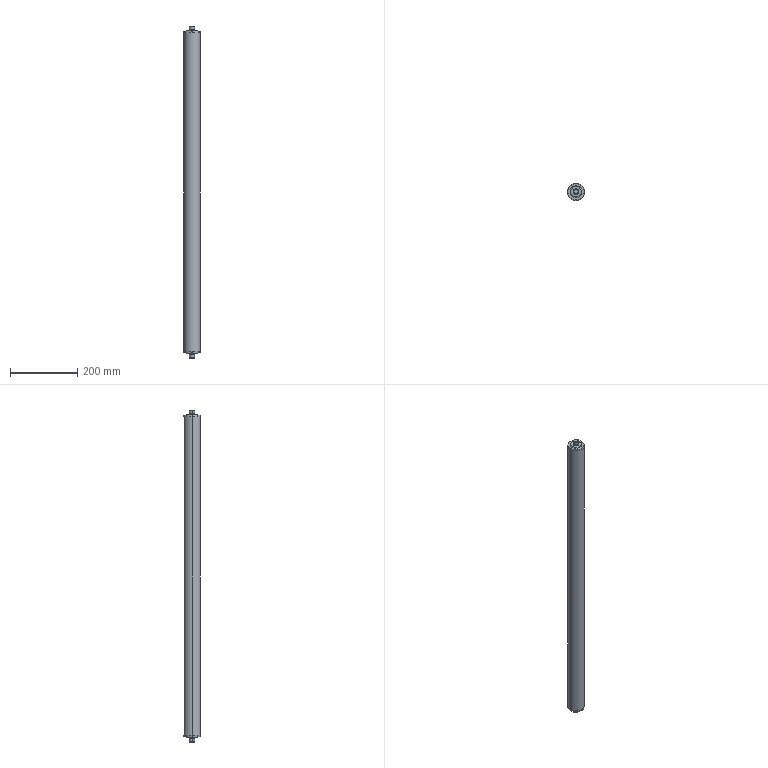Part | SolidWorks | features Chamfer 2, ICE 2, Revolution 1 | 1 solid | 30 faces | box 50 x 50 x 985 mm | volume 1880684 mm3 | cone 12 | cylinder 10 | plane 8 | commonest cylinder face diameters 15 x4 17 x4 50 x2
STEP:
#1=CARTESIAN_POINT('',(6.5,0.,340.5));
#2=VERTEX_POINT('',#1);
#3=CARTESIAN_POINT('',(-6.5,0.,340.5));
#4=VERTEX_POINT('',#3);
#5=CARTESIAN_POINT('',(0.,0.,340.5));
#6=DIRECTION('',(0.,0.,1.));
#7=DIRECTION('',(-1.,0.,0.));
#8=AXIS2_PLACEMENT_3D('',#5,#6,#7);
#9=CIRCLE('',#8,6.5);
#10=EDGE_CURVE('',#2,#4,#9,.T.);
#11=ORIENTED_EDGE('',*,*,#10,.F.);
#12=CARTESIAN_POINT('',(7.5,0.,339.5));
#13=VERTEX_POINT('',#12);
#14=CARTESIAN_POINT('',(6.5,0.,340.5));
#15=DIRECTION('',(0.7071,0.,-0.7071));
#16=VECTOR('',#15,1000.);
#17=LINE('',#14,#16);
#18=EDGE_CURVE('',#2,#13,#17,.T.);
#19=ORIENTED_EDGE('',*,*,#18,.T.);
#20=CARTESIAN_POINT('',(-7.5,0.,339.5));
#21=VERTEX_POINT('',#20);
#22=CARTESIAN_POINT('',(0.,0.,339.5));
#23=DIRECTION('',(0.,0.,-1.));
#24=DIRECTION('',(-1.,0.,0.));
#25=AXIS2_PLACEMENT_3D('',#22,#23,#24);
#26=CIRCLE('',#25,7.5);
#27=EDGE_CURVE('',#21,#13,#26,.T.);
#28=ORIENTED_EDGE('',*,*,#27,.F.);
#29=CARTESIAN_POINT('',(-6.5,0.,340.5));
#30=DIRECTION('',(-0.7071,0.,-0.7071));
#31=VECTOR('',#30,1000.);
#32=LINE('',#29,#31);
#33=EDGE_CURVE('',#4,#21,#32,.T.);
#34=ORIENTED_EDGE('',*,*,#33,.F.);
#35=EDGE_LOOP('',(#11,#19,#28,#34));
#36=FACE_OUTER_BOUND('',#35,.T.);
#37=CARTESIAN_POINT('',(0.,0.,340.5));
#38=DIRECTION('',(0.,0.,-1.));
#39=DIRECTION('',(-1.,0.,0.));
#40=AXIS2_PLACEMENT_3D('',#37,#38,#39);
#41=CONICAL_SURFACE('',#40,6.5,0.7854);
#42=ADVANCED_FACE('',(#36),#41,.T.);
#43=CARTESIAN_POINT('',(-6.5,0.,-644.5));
#44=VERTEX_POINT('',#43);
#45=CARTESIAN_POINT('',(6.5,0.,-644.5));
#46=VERTEX_POINT('',#45);
#47=CARTESIAN_POINT('',(0.,0.,-644.5));
#48=DIRECTION('',(0.,0.,-1.));
#49=DIRECTION('',(1.,0.,0.));
#50=AXIS2_PLACEMENT_3D('',#47,#48,#49);
#51=CIRCLE('',#50,6.5);
#52=EDGE_CURVE('',#44,#46,#51,.T.);
#53=ORIENTED_EDGE('',*,*,#52,.F.);
#54=CARTESIAN_POINT('',(-7.5,0.,-643.5));
#55=VERTEX_POINT('',#54);
#56=CARTESIAN_POINT('',(-7.5,0.,-643.5));
#57=DIRECTION('',(-0.7071,0.,0.7071));
#58=VECTOR('',#57,1000.);
#59=LINE('',#56,#58);
#60=EDGE_CURVE('',#44,#55,#59,.T.);
#61=ORIENTED_EDGE('',*,*,#60,.T.);
#62=CARTESIAN_POINT('',(7.5,0.,-643.5));
#63=VERTEX_POINT('',#62);
#64=CARTESIAN_POINT('',(0.,0.,-643.5));
#65=DIRECTION('',(0.,0.,1.));
#66=DIRECTION('',(1.,0.,0.));
#67=AXIS2_PLACEMENT_3D('',#64,#65,#66);
#68=CIRCLE('',#67,7.5);
#69=EDGE_CURVE('',#63,#55,#68,.T.);
#70=ORIENTED_EDGE('',*,*,#69,.F.);
#71=CARTESIAN_POINT('',(7.5,0.,-643.5));
#72=DIRECTION('',(0.7071,0.,0.7071));
#73=VECTOR('',#72,1000.);
#74=LINE('',#71,#73);
#75=EDGE_CURVE('',#46,#63,#74,.T.);
#76=ORIENTED_EDGE('',*,*,#75,.F.);
#77=EDGE_LOOP('',(#53,#61,#70,#76));
#78=FACE_OUTER_BOUND('',#77,.T.);
#79=CARTESIAN_POINT('',(0.,0.,-643.5));
#80=DIRECTION('',(0.,0.,1.));
#81=DIRECTION('',(1.,0.,0.));
#82=AXIS2_PLACEMENT_3D('',#79,#80,#81);
#83=CONICAL_SURFACE('',#82,7.5,0.7854);
#84=ADVANCED_FACE('',(#78),#83,.T.);
#85=CARTESIAN_POINT('',(24.118,0.,325.));
#86=VERTEX_POINT('',#85);
#87=CARTESIAN_POINT('',(-24.118,0.,325.));
#88=VERTEX_POINT('',#87);
#89=CARTESIAN_POINT('',(0.,0.,325.));
#90=DIRECTION('',(0.,0.,1.));
#91=DIRECTION('',(-1.,0.,0.));
#92=AXIS2_PLACEMENT_3D('',#89,#90,#91);
#93=CIRCLE('',#92,24.118);
#94=EDGE_CURVE('',#86,#88,#93,.T.);
#95=ORIENTED_EDGE('',*,*,#94,.F.);
#96=CARTESIAN_POINT('',(25.,0.,320.));
#97=VERTEX_POINT('',#96);
#98=CARTESIAN_POINT('',(24.118,0.,325.));
#99=DIRECTION('',(0.1736,0.,-0.9848));
#100=VECTOR('',#99,1000.);
#101=LINE('',#98,#100);
#102=EDGE_CURVE('',#86,#97,#101,.T.);
#103=ORIENTED_EDGE('',*,*,#102,.T.);
#104=CARTESIAN_POINT('',(-25.,0.,320.));
#105=VERTEX_POINT('',#104);
#106=CARTESIAN_POINT('',(0.,0.,320.));
#107=DIRECTION('',(0.,0.,-1.));
#108=DIRECTION('',(-1.,0.,0.));
#109=AXIS2_PLACEMENT_3D('',#106,#107,#108);
#110=CIRCLE('',#109,25.);
#111=EDGE_CURVE('',#105,#97,#110,.T.);
#112=ORIENTED_EDGE('',*,*,#111,.F.);
#113=CARTESIAN_POINT('',(-24.118,0.,325.));
#114=DIRECTION('',(-0.1736,0.,-0.9848));
#115=VECTOR('',#114,1000.);
#116=LINE('',#113,#115);
#117=EDGE_CURVE('',#88,#105,#116,.T.);
#118=ORIENTED_EDGE('',*,*,#117,.F.);
#119=EDGE_LOOP('',(#95,#103,#112,#118));
#120=FACE_OUTER_BOUND('',#119,.T.);
#121=CARTESIAN_POINT('',(0.,0.,325.));
#122=DIRECTION('',(0.,0.,-1.));
#123=DIRECTION('',(-1.,0.,0.));
#124=AXIS2_PLACEMENT_3D('',#121,#122,#123);
#125=CONICAL_SURFACE('',#124,24.118,0.1745);
#126=ADVANCED_FACE('',(#120),#125,.T.);
#127=CARTESIAN_POINT('',(-24.118,0.,-629.));
#128=VERTEX_POINT('',#127);
#129=CARTESIAN_POINT('',(24.118,0.,-629.));
#130=VERTEX_POINT('',#129);
#131=CARTESIAN_POINT('',(0.,0.,-629.));
#132=DIRECTION('',(0.,0.,-1.));
#133=DIRECTION('',(1.,0.,0.));
#134=AXIS2_PLACEMENT_3D('',#131,#132,#133);
#135=CIRCLE('',#134,24.118);
#136=EDGE_CURVE('',#128,#130,#135,.T.);
#137=ORIENTED_EDGE('',*,*,#136,.F.);
#138=CARTESIAN_POINT('',(-25.,0.,-624.));
#139=VERTEX_POINT('',#138);
#140=CARTESIAN_POINT('',(-25.,0.,-624.));
#141=DIRECTION('',(-0.1736,0.,0.9848));
#142=VECTOR('',#141,1000.);
#143=LINE('',#140,#142);
#144=EDGE_CURVE('',#128,#139,#143,.T.);
#145=ORIENTED_EDGE('',*,*,#144,.T.);
#146=CARTESIAN_POINT('',(25.,0.,-624.));
#147=VERTEX_POINT('',#146);
#148=CARTESIAN_POINT('',(0.,0.,-624.));
#149=DIRECTION('',(0.,0.,1.));
#150=DIRECTION('',(1.,0.,0.));
#151=AXIS2_PLACEMENT_3D('',#148,#149,#150);
#152=CIRCLE('',#151,25.);
#153=EDGE_CURVE('',#147,#139,#152,.T.);
#154=ORIENTED_EDGE('',*,*,#153,.F.);
#155=CARTESIAN_POINT('',(25.,0.,-624.));
#156=DIRECTION('',(0.1736,0.,0.9848));
#157=VECTOR('',#156,1000.);
#158=LINE('',#155,#157);
#159=EDGE_CURVE('',#130,#147,#158,.T.);
#160=ORIENTED_EDGE('',*,*,#159,.F.);
#161=EDGE_LOOP('',(#137,#145,#154,#160));
#162=FACE_OUTER_BOUND('',#161,.T.);
#163=CARTESIAN_POINT('',(0.,0.,-624.));
#164=DIRECTION('',(0.,0.,1.));
#165=DIRECTION('',(1.,0.,0.));
#166=AXIS2_PLACEMENT_3D('',#163,#164,#165);
#167=CONICAL_SURFACE('',#166,25.,0.1745);
#168=ADVANCED_FACE('',(#162),#167,.T.);
#169=CARTESIAN_POINT('',(15.701,0.,326.761));
#170=VERTEX_POINT('',#169);
#171=CARTESIAN_POINT('',(-15.701,0.,326.761));
#172=VERTEX_POINT('',#171);
#173=CARTESIAN_POINT('',(0.,0.,326.761));
#174=DIRECTION('',(0.,0.,1.));
#175=DIRECTION('',(1.,0.,0.));
#176=AXIS2_PLACEMENT_3D('',#173,#174,#175);
#177=CIRCLE('',#176,15.701);
#178=EDGE_CURVE('',#170,#172,#177,.T.);
#179=ORIENTED_EDGE('',*,*,#178,.F.);
#180=CARTESIAN_POINT('',(17.799,0.,325.));
#181=VERTEX_POINT('',#180);
#182=CARTESIAN_POINT('',(17.799,0.,325.));
#183=DIRECTION('',(0.766,0.,-0.6428));
#184=VECTOR('',#183,1000.);
#185=LINE('',#182,#184);
#186=EDGE_CURVE('',#170,#181,#185,.T.);
#187=ORIENTED_EDGE('',*,*,#186,.T.);
#188=CARTESIAN_POINT('',(-17.799,0.,325.));
#189=VERTEX_POINT('',#188);
#190=CARTESIAN_POINT('',(0.,0.,325.));
#191=DIRECTION('',(0.,0.,1.));
#192=DIRECTION('',(1.,0.,0.));
#193=AXIS2_PLACEMENT_3D('',#190,#191,#192);
#194=CIRCLE('',#193,17.799);
#195=EDGE_CURVE('',#181,#189,#194,.T.);
#196=ORIENTED_EDGE('',*,*,#195,.T.);
#197=CARTESIAN_POINT('',(-17.799,0.,325.));
#198=DIRECTION('',(-0.766,0.,-0.6428));
#199=VECTOR('',#198,1000.);
#200=LINE('',#197,#199);
#201=EDGE_CURVE('',#172,#189,#200,.T.);
#202=ORIENTED_EDGE('',*,*,#201,.F.);
#203=EDGE_LOOP('',(#179,#187,#196,#202));
#204=FACE_OUTER_BOUND('',#203,.T.);
#205=CARTESIAN_POINT('',(0.,0.,325.));
#206=DIRECTION('',(0.,0.,-1.));
#207=DIRECTION('',(-1.,0.,0.));
#208=AXIS2_PLACEMENT_3D('',#205,#206,#207);
#209=CONICAL_SURFACE('',#208,17.799,0.8727);
#210=ADVANCED_FACE('',(#204),#209,.T.);
#211=CARTESIAN_POINT('',(8.5,0.,326.761));
#212=VERTEX_POINT('',#211);
#213=CARTESIAN_POINT('',(-8.5,0.,326.761));
#214=VERTEX_POINT('',#213);
#215=CARTESIAN_POINT('',(0.,0.,326.761));
#216=DIRECTION('',(0.,0.,1.));
#217=DIRECTION('',(1.,0.,0.));
#218=AXIS2_PLACEMENT_3D('',#215,#216,#217);
#219=CIRCLE('',#218,8.5);
#220=EDGE_CURVE('',#212,#214,#219,.T.);
#221=ORIENTED_EDGE('',*,*,#220,.T.);
#222=CARTESIAN_POINT('',(-8.5,0.,329.5));
#223=VERTEX_POINT('',#222);
#224=CARTESIAN_POINT('',(-8.5,0.,340.5));
#225=DIRECTION('',(0.,0.,1.));
#226=VECTOR('',#225,1000.);
#227=LINE('',#224,#226);
#228=EDGE_CURVE('',#214,#223,#227,.T.);
#229=ORIENTED_EDGE('',*,*,#228,.T.);
#230=CARTESIAN_POINT('',(8.5,0.,329.5));
#231=VERTEX_POINT('',#230);
#232=CARTESIAN_POINT('',(0.,0.,329.5));
#233=DIRECTION('',(0.,0.,1.));
#234=DIRECTION('',(1.,0.,0.));
#235=AXIS2_PLACEMENT_3D('',#232,#233,#234);
#236=CIRCLE('',#235,8.5);
#237=EDGE_CURVE('',#231,#223,#236,.T.);
#238=ORIENTED_EDGE('',*,*,#237,.F.);
#239=CARTESIAN_POINT('',(8.5,0.,340.5));
#240=DIRECTION('',(0.,0.,1.));
#241=VECTOR('',#240,1000.);
#242=LINE('',#239,#241);
#243=EDGE_CURVE('',#212,#231,#242,.T.);
#244=ORIENTED_EDGE('',*,*,#243,.F.);
#245=EDGE_LOOP('',(#221,#229,#238,#244));
#246=FACE_OUTER_BOUND('',#245,.T.);
#247=CARTESIAN_POINT('',(0.,0.,340.5));
#248=DIRECTION('',(0.,0.,1.));
#249=DIRECTION('',(1.,0.,0.));
#250=AXIS2_PLACEMENT_3D('',#247,#248,#249);
#251=CYLINDRICAL_SURFACE('',#250,8.5);
#252=ADVANCED_FACE('',(#246),#251,.T.);
#253=CARTESIAN_POINT('',(7.5,0.,329.5));
#254=VERTEX_POINT('',#253);
#255=CARTESIAN_POINT('',(-7.5,0.,329.5));
#256=VERTEX_POINT('',#255);
#257=CARTESIAN_POINT('',(0.,0.,329.5));
#258=DIRECTION('',(0.,0.,1.));
#259=DIRECTION('',(1.,0.,0.));
#260=AXIS2_PLACEMENT_3D('',#257,#258,#259);
#261=CIRCLE('',#260,7.5);
#262=EDGE_CURVE('',#254,#256,#261,.T.);
#263=ORIENTED_EDGE('',*,*,#262,.T.);
#264=CARTESIAN_POINT('',(-7.5,0.,340.5));
#265=DIRECTION('',(0.,0.,1.));
#266=VECTOR('',#265,1000.);
#267=LINE('',#264,#266);
#268=EDGE_CURVE('',#256,#21,#267,.T.);
#269=ORIENTED_EDGE('',*,*,#268,.T.);
#270=ORIENTED_EDGE('',*,*,#27,.T.);
#271=CARTESIAN_POINT('',(7.5,0.,340.5));
#272=DIRECTION('',(0.,0.,1.));
#273=VECTOR('',#272,1000.);
#274=LINE('',#271,#273);
#275=EDGE_CURVE('',#254,#13,#274,.T.);
#276=ORIENTED_EDGE('',*,*,#275,.F.);
#277=EDGE_LOOP('',(#263,#269,#270,#276));
#278=FACE_OUTER_BOUND('',#277,.T.);
#279=CARTESIAN_POINT('',(0.,0.,340.5));
#280=DIRECTION('',(0.,0.,1.));
#281=DIRECTION('',(1.,0.,0.));
#282=AXIS2_PLACEMENT_3D('',#279,#280,#281);
#283=CYLINDRICAL_SURFACE('',#282,7.5);
#284=ADVANCED_FACE('',(#278),#283,.T.);
#285=ORIENTED_EDGE('',*,*,#69,.T.);
#286=CARTESIAN_POINT('',(-7.5,0.,-633.5));
#287=VERTEX_POINT('',#286);
#288=CARTESIAN_POINT('',(-7.5,0.,340.5));
#289=DIRECTION('',(0.,0.,1.));
#290=VECTOR('',#289,1000.);
#291=LINE('',#288,#290);
#292=EDGE_CURVE('',#55,#287,#291,.T.);
#293=ORIENTED_EDGE('',*,*,#292,.T.);
#294=CARTESIAN_POINT('',(7.5,0.,-633.5));
#295=VERTEX_POINT('',#294);
#296=CARTESIAN_POINT('',(0.,0.,-633.5));
#297=DIRECTION('',(0.,0.,1.));
#298=DIRECTION('',(1.,0.,0.));
#299=AXIS2_PLACEMENT_3D('',#296,#297,#298);
#300=CIRCLE('',#299,7.5);
#301=EDGE_CURVE('',#295,#287,#300,.T.);
#302=ORIENTED_EDGE('',*,*,#301,.F.);
#303=CARTESIAN_POINT('',(7.5,0.,340.5));
#304=DIRECTION('',(0.,0.,1.));
#305=VECTOR('',#304,1000.);
#306=LINE('',#303,#305);
#307=EDGE_CURVE('',#63,#295,#306,.T.);
#308=ORIENTED_EDGE('',*,*,#307,.F.);
#309=EDGE_LOOP('',(#285,#293,#302,#308));
#310=FACE_OUTER_BOUND('',#309,.T.);
#311=CARTESIAN_POINT('',(0.,0.,340.5));
#312=DIRECTION('',(0.,0.,1.));
#313=DIRECTION('',(1.,0.,0.));
#314=AXIS2_PLACEMENT_3D('',#311,#312,#313);
#315=CYLINDRICAL_SURFACE('',#314,7.5);
#316=ADVANCED_FACE('',(#310),#315,.T.);
#317=CARTESIAN_POINT('',(8.5,0.,-633.5));
#318=VERTEX_POINT('',#317);
#319=CARTESIAN_POINT('',(-8.5,0.,-633.5));
#320=VERTEX_POINT('',#319);
#321=CARTESIAN_POINT('',(0.,0.,-633.5));
#322=DIRECTION('',(0.,0.,1.));
#323=DIRECTION('',(1.,0.,0.));
#324=AXIS2_PLACEMENT_3D('',#321,#322,#323);
#325=CIRCLE('',#324,8.5);
#326=EDGE_CURVE('',#318,#320,#325,.T.);
#327=ORIENTED_EDGE('',*,*,#326,.T.);
#328=CARTESIAN_POINT('',(-8.5,0.,-630.761));
#329=VERTEX_POINT('',#328);
#330=CARTESIAN_POINT('',(-8.5,0.,340.5));
#331=DIRECTION('',(0.,0.,1.));
#332=VECTOR('',#331,1000.);
#333=LINE('',#330,#332);
#334=EDGE_CURVE('',#320,#329,#333,.T.);
#335=ORIENTED_EDGE('',*,*,#334,.T.);
#336=CARTESIAN_POINT('',(8.5,0.,-630.761));
#337=VERTEX_POINT('',#336);
#338=CARTESIAN_POINT('',(0.,0.,-630.761));
#339=DIRECTION('',(0.,0.,1.));
#340=DIRECTION('',(1.,0.,0.));
#341=AXIS2_PLACEMENT_3D('',#338,#339,#340);
#342=CIRCLE('',#341,8.5);
#343=EDGE_CURVE('',#337,#329,#342,.T.);
#344=ORIENTED_EDGE('',*,*,#343,.F.);
#345=CARTESIAN_POINT('',(8.5,0.,340.5));
#346=DIRECTION('',(0.,0.,1.));
#347=VECTOR('',#346,1000.);
#348=LINE('',#345,#347);
#349=EDGE_CURVE('',#318,#337,#348,.T.);
#350=ORIENTED_EDGE('',*,*,#349,.F.);
#351=EDGE_LOOP('',(#327,#335,#344,#350));
#352=FACE_OUTER_BOUND('',#351,.T.);
#353=CARTESIAN_POINT('',(0.,0.,340.5));
#354=DIRECTION('',(0.,0.,1.));
#355=DIRECTION('',(1.,0.,0.));
#356=AXIS2_PLACEMENT_3D('',#353,#354,#355);
#357=CYLINDRICAL_SURFACE('',#356,8.5);
#358=ADVANCED_FACE('',(#352),#357,.T.);
#359=CARTESIAN_POINT('',(15.701,0.,-630.761));
#360=VERTEX_POINT('',#359);
#361=CARTESIAN_POINT('',(-15.701,0.,-630.761));
#362=VERTEX_POINT('',#361);
#363=CARTESIAN_POINT('',(0.,0.,-630.761));
#364=DIRECTION('',(0.,0.,1.));
#365=DIRECTION('',(1.,0.,0.));
#366=AXIS2_PLACEMENT_3D('',#363,#364,#365);
#367=CIRCLE('',#366,15.701);
#368=EDGE_CURVE('',#360,#362,#367,.T.);
#369=ORIENTED_EDGE('',*,*,#368,.T.);
#370=CARTESIAN_POINT('',(-17.799,0.,-629.));
#371=VERTEX_POINT('',#370);
#372=CARTESIAN_POINT('',(-15.701,0.,-630.761));
#373=DIRECTION('',(-0.766,0.,0.6428));
#374=VECTOR('',#373,1000.);
#375=LINE('',#372,#374);
#376=EDGE_CURVE('',#362,#371,#375,.T.);
#377=ORIENTED_EDGE('',*,*,#376,.T.);
#378=CARTESIAN_POINT('',(17.799,0.,-629.));
#379=VERTEX_POINT('',#378);
#380=CARTESIAN_POINT('',(0.,0.,-629.));
#381=DIRECTION('',(0.,0.,1.));
#382=DIRECTION('',(1.,0.,0.));
#383=AXIS2_PLACEMENT_3D('',#380,#381,#382);
#384=CIRCLE('',#383,17.799);
#385=EDGE_CURVE('',#379,#371,#384,.T.);
#386=ORIENTED_EDGE('',*,*,#385,.F.);
#387=CARTESIAN_POINT('',(15.701,0.,-630.761));
#388=DIRECTION('',(0.766,0.,0.6428));
#389=VECTOR('',#388,1000.);
#390=LINE('',#387,#389);
#391=EDGE_CURVE('',#360,#379,#390,.T.);
#392=ORIENTED_EDGE('',*,*,#391,.F.);
#393=EDGE_LOOP('',(#369,#377,#386,#392));
#394=FACE_OUTER_BOUND('',#393,.T.);
#395=CARTESIAN_POINT('',(0.,0.,-630.761));
#396=DIRECTION('',(0.,0.,1.));
#397=DIRECTION('',(1.,0.,0.));
#398=AXIS2_PLACEMENT_3D('',#395,#396,#397);
#399=CONICAL_SURFACE('',#398,15.701,0.8727);
#400=ADVANCED_FACE('',(#394),#399,.T.);
#401=ORIENTED_EDGE('',*,*,#153,.T.);
#402=CARTESIAN_POINT('',(-25.,0.,340.5));
#403=DIRECTION('',(0.,0.,1.));
#404=VECTOR('',#403,1000.);
#405=LINE('',#402,#404);
#406=EDGE_CURVE('',#139,#105,#405,.T.);
#407=ORIENTED_EDGE('',*,*,#406,.T.);
#408=ORIENTED_EDGE('',*,*,#111,.T.);
#409=CARTESIAN_POINT('',(25.,0.,340.5));
#410=DIRECTION('',(0.,0.,1.));
#411=VECTOR('',#410,1000.);
#412=LINE('',#409,#411);
#413=EDGE_CURVE('',#147,#97,#412,.T.);
#414=ORIENTED_EDGE('',*,*,#413,.F.);
#415=EDGE_LOOP('',(#401,#407,#408,#414));
#416=FACE_OUTER_BOUND('',#415,.T.);
#417=CARTESIAN_POINT('',(0.,0.,340.5));
#418=DIRECTION('',(0.,0.,1.));
#419=DIRECTION('',(1.,0.,0.));
#420=AXIS2_PLACEMENT_3D('',#417,#418,#419);
#421=CYLINDRICAL_SURFACE('',#420,25.);
#422=ADVANCED_FACE('',(#416),#421,.T.);
#423=CARTESIAN_POINT('',(0.,0.,325.));
#424=DIRECTION('',(0.,0.,1.));
#425=DIRECTION('',(-1.,0.,0.));
#426=AXIS2_PLACEMENT_3D('',#423,#424,#425);
#427=CIRCLE('',#426,24.118);
#428=EDGE_CURVE('',#88,#86,#427,.T.);
#429=ORIENTED_EDGE('',*,*,#428,.T.);
#430=ORIENTED_EDGE('',*,*,#94,.T.);
#431=EDGE_LOOP('',(#429,#430));
#432=FACE_OUTER_BOUND('',#431,.T.);
#433=CARTESIAN_POINT('',(0.,0.,325.));
#434=DIRECTION('',(0.,0.,1.));
#435=DIRECTION('',(1.,0.,0.));
#436=AXIS2_PLACEMENT_3D('',#433,#434,#435);
#437=CIRCLE('',#436,17.799);
#438=EDGE_CURVE('',#189,#181,#437,.T.);
#439=ORIENTED_EDGE('',*,*,#438,.F.);
#440=ORIENTED_EDGE('',*,*,#195,.F.);
#441=EDGE_LOOP('',(#439,#440));
#442=FACE_BOUND('',#441,.T.);
#443=CARTESIAN_POINT('',(0.,17.799,325.));
#444=DIRECTION('',(0.,0.,-1.));
#445=DIRECTION('',(-1.,0.,0.));
#446=AXIS2_PLACEMENT_3D('',#443,#444,#445);
#447=PLANE('',#446);
#448=ADVANCED_FACE('',(#432,#442),#447,.F.);
#449=ORIENTED_EDGE('',*,*,#406,.F.);
#450=CARTESIAN_POINT('',(0.,0.,-624.));
#451=DIRECTION('',(0.,0.,1.));
#452=DIRECTION('',(1.,0.,0.));
#453=AXIS2_PLACEMENT_3D('',#450,#451,#452);
#454=CIRCLE('',#453,25.);
#455=EDGE_CURVE('',#139,#147,#454,.T.);
#456=ORIENTED_EDGE('',*,*,#455,.T.);
#457=ORIENTED_EDGE('',*,*,#413,.T.);
#458=CARTESIAN_POINT('',(0.,0.,320.));
#459=DIRECTION('',(0.,0.,-1.));
#460=DIRECTION('',(-1.,0.,0.));
#461=AXIS2_PLACEMENT_3D('',#458,#459,#460);
#462=CIRCLE('',#461,25.);
#463=EDGE_CURVE('',#97,#105,#462,.T.);
#464=ORIENTED_EDGE('',*,*,#463,.T.);
#465=EDGE_LOOP('',(#449,#456,#457,#464));
#466=FACE_OUTER_BOUND('',#465,.T.);
#467=CARTESIAN_POINT('',(0.,0.,340.5));
#468=DIRECTION('',(0.,0.,1.));
#469=DIRECTION('',(1.,0.,0.));
#470=AXIS2_PLACEMENT_3D('',#467,#468,#469);
#471=CYLINDRICAL_SURFACE('',#470,25.);
#472=ADVANCED_FACE('',(#466),#471,.T.);
#473=CARTESIAN_POINT('',(0.,0.,-629.));
#474=DIRECTION('',(0.,0.,-1.));
#475=DIRECTION('',(1.,0.,0.));
#476=AXIS2_PLACEMENT_3D('',#473,#474,#475);
#477=CIRCLE('',#476,24.118);
#478=EDGE_CURVE('',#130,#128,#477,.T.);
#479=ORIENTED_EDGE('',*,*,#478,.T.);
#480=ORIENTED_EDGE('',*,*,#136,.T.);
#481=EDGE_LOOP('',(#479,#480));
#482=FACE_OUTER_BOUND('',#481,.T.);
#483=ORIENTED_EDGE('',*,*,#385,.T.);
#484=CARTESIAN_POINT('',(0.,0.,-629.));
#485=DIRECTION('',(0.,0.,1.));
#486=DIRECTION('',(1.,0.,0.));
#487=AXIS2_PLACEMENT_3D('',#484,#485,#486);
#488=CIRCLE('',#487,17.799);
#489=EDGE_CURVE('',#371,#379,#488,.T.);
#490=ORIENTED_EDGE('',*,*,#489,.T.);
#491=EDGE_LOOP('',(#483,#490));
#492=FACE_BOUND('',#491,.T.);
#493=CARTESIAN_POINT('',(0.,17.799,-629.));
#494=DIRECTION('',(0.,0.,1.));
#495=DIRECTION('',(1.,0.,0.));
#496=AXIS2_PLACEMENT_3D('',#493,#494,#495);
#497=PLANE('',#496);
#498=ADVANCED_FACE('',(#482,#492),#497,.F.);
#499=ORIENTED_EDGE('',*,*,#376,.F.);
#500=CARTESIAN_POINT('',(0.,0.,-630.761));
#501=DIRECTION('',(0.,0.,1.));
#502=DIRECTION('',(1.,0.,0.));
#503=AXIS2_PLACEMENT_3D('',#500,#501,#502);
#504=CIRCLE('',#503,15.701);
#505=EDGE_CURVE('',#362,#360,#504,.T.);
#506=ORIENTED_EDGE('',*,*,#505,.T.);
#507=ORIENTED_EDGE('',*,*,#391,.T.);
#508=ORIENTED_EDGE('',*,*,#489,.F.);
#509=EDGE_LOOP('',(#499,#506,#507,#508));
#510=FACE_OUTER_BOUND('',#509,.T.);
#511=CARTESIAN_POINT('',(0.,0.,-630.761));
#512=DIRECTION('',(0.,0.,1.));
#513=DIRECTION('',(1.,0.,0.));
#514=AXIS2_PLACEMENT_3D('',#511,#512,#513);
#515=CONICAL_SURFACE('',#514,15.701,0.8727);
#516=ADVANCED_FACE('',(#510),#515,.T.);
#517=ORIENTED_EDGE('',*,*,#368,.F.);
#518=ORIENTED_EDGE('',*,*,#505,.F.);
#519=EDGE_LOOP('',(#517,#518));
#520=FACE_OUTER_BOUND('',#519,.T.);
#521=ORIENTED_EDGE('',*,*,#343,.T.);
#522=CARTESIAN_POINT('',(0.,0.,-630.761));
#523=DIRECTION('',(0.,0.,1.));
#524=DIRECTION('',(1.,0.,0.));
#525=AXIS2_PLACEMENT_3D('',#522,#523,#524);
#526=CIRCLE('',#525,8.5);
#527=EDGE_CURVE('',#329,#337,#526,.T.);
#528=ORIENTED_EDGE('',*,*,#527,.T.);
#529=EDGE_LOOP('',(#521,#528));
#530=FACE_BOUND('',#529,.T.);
#531=CARTESIAN_POINT('',(0.,8.5,-630.761));
#532=DIRECTION('',(0.,0.,1.));
#533=DIRECTION('',(1.,0.,0.));
#534=AXIS2_PLACEMENT_3D('',#531,#532,#533);
#535=PLANE('',#534);
#536=ADVANCED_FACE('',(#520,#530),#535,.F.);
#537=ORIENTED_EDGE('',*,*,#334,.F.);
#538=CARTESIAN_POINT('',(0.,0.,-633.5));
#539=DIRECTION('',(0.,0.,1.));
#540=DIRECTION('',(1.,0.,0.));
#541=AXIS2_PLACEMENT_3D('',#538,#539,#540);
#542=CIRCLE('',#541,8.5);
#543=EDGE_CURVE('',#320,#318,#542,.T.);
#544=ORIENTED_EDGE('',*,*,#543,.T.);
#545=ORIENTED_EDGE('',*,*,#349,.T.);
#546=ORIENTED_EDGE('',*,*,#527,.F.);
#547=EDGE_LOOP('',(#537,#544,#545,#546));
#548=FACE_OUTER_BOUND('',#547,.T.);
#549=CARTESIAN_POINT('',(0.,0.,340.5));
#550=DIRECTION('',(0.,0.,1.));
#551=DIRECTION('',(1.,0.,0.));
#552=AXIS2_PLACEMENT_3D('',#549,#550,#551);
#553=CYLINDRICAL_SURFACE('',#552,8.5);
#554=ADVANCED_FACE('',(#548),#553,.T.);
#555=ORIENTED_EDGE('',*,*,#326,.F.);
#556=ORIENTED_EDGE('',*,*,#543,.F.);
#557=EDGE_LOOP('',(#555,#556));
#558=FACE_OUTER_BOUND('',#557,.T.);
#559=ORIENTED_EDGE('',*,*,#301,.T.);
#560=CARTESIAN_POINT('',(0.,0.,-633.5));
#561=DIRECTION('',(0.,0.,1.));
#562=DIRECTION('',(1.,0.,0.));
#563=AXIS2_PLACEMENT_3D('',#560,#561,#562);
#564=CIRCLE('',#563,7.5);
#565=EDGE_CURVE('',#287,#295,#564,.T.);
#566=ORIENTED_EDGE('',*,*,#565,.T.);
#567=EDGE_LOOP('',(#559,#566));
#568=FACE_BOUND('',#567,.T.);
#569=CARTESIAN_POINT('',(0.,7.5,-633.5));
#570=DIRECTION('',(0.,0.,1.));
#571=DIRECTION('',(1.,0.,0.));
#572=AXIS2_PLACEMENT_3D('',#569,#570,#571);
#573=PLANE('',#572);
#574=ADVANCED_FACE('',(#558,#568),#573,.F.);
#575=ORIENTED_EDGE('',*,*,#292,.F.);
#576=CARTESIAN_POINT('',(0.,0.,-643.5));
#577=DIRECTION('',(0.,0.,1.));
#578=DIRECTION('',(1.,0.,0.));
#579=AXIS2_PLACEMENT_3D('',#576,#577,#578);
#580=CIRCLE('',#579,7.5);
#581=EDGE_CURVE('',#55,#63,#580,.T.);
#582=ORIENTED_EDGE('',*,*,#581,.T.);
#583=ORIENTED_EDGE('',*,*,#307,.T.);
#584=ORIENTED_EDGE('',*,*,#565,.F.);
#585=EDGE_LOOP('',(#575,#582,#583,#584));
#586=FACE_OUTER_BOUND('',#585,.T.);
#587=CARTESIAN_POINT('',(0.,0.,340.5));
#588=DIRECTION('',(0.,0.,1.));
#589=DIRECTION('',(1.,0.,0.));
#590=AXIS2_PLACEMENT_3D('',#587,#588,#589);
#591=CYLINDRICAL_SURFACE('',#590,7.5);
#592=ADVANCED_FACE('',(#586),#591,.T.);
#593=CARTESIAN_POINT('',(0.,0.,-644.5));
#594=DIRECTION('',(0.,0.,-1.));
#595=DIRECTION('',(1.,0.,0.));
#596=AXIS2_PLACEMENT_3D('',#593,#594,#595);
#597=CIRCLE('',#596,6.5);
#598=EDGE_CURVE('',#46,#44,#597,.T.);
#599=ORIENTED_EDGE('',*,*,#598,.T.);
#600=ORIENTED_EDGE('',*,*,#52,.T.);
#601=EDGE_LOOP('',(#599,#600));
#602=FACE_OUTER_BOUND('',#601,.T.);
#603=CARTESIAN_POINT('',(0.,0.,-644.5));
#604=DIRECTION('',(0.,0.,1.));
#605=DIRECTION('',(1.,0.,0.));
#606=AXIS2_PLACEMENT_3D('',#603,#604,#605);
#607=PLANE('',#606);
#608=ADVANCED_FACE('',(#602),#607,.F.);
#609=CARTESIAN_POINT('',(0.,0.,340.5));
#610=DIRECTION('',(0.,0.,1.));
#611=DIRECTION('',(-1.,0.,0.));
#612=AXIS2_PLACEMENT_3D('',#609,#610,#611);
#613=CIRCLE('',#612,6.5);
#614=EDGE_CURVE('',#4,#2,#613,.T.);
#615=ORIENTED_EDGE('',*,*,#614,.T.);
#616=ORIENTED_EDGE('',*,*,#10,.T.);
#617=EDGE_LOOP('',(#615,#616));
#618=FACE_OUTER_BOUND('',#617,.T.);
#619=CARTESIAN_POINT('',(0.,0.,340.5));
#620=DIRECTION('',(0.,0.,-1.));
#621=DIRECTION('',(-1.,0.,0.));
#622=AXIS2_PLACEMENT_3D('',#619,#620,#621);
#623=PLANE('',#622);
#624=ADVANCED_FACE('',(#618),#623,.F.);
#625=ORIENTED_EDGE('',*,*,#268,.F.);
#626=CARTESIAN_POINT('',(0.,0.,329.5));
#627=DIRECTION('',(0.,0.,1.));
#628=DIRECTION('',(1.,0.,0.));
#629=AXIS2_PLACEMENT_3D('',#626,#627,#628);
#630=CIRCLE('',#629,7.5);
#631=EDGE_CURVE('',#256,#254,#630,.T.);
#632=ORIENTED_EDGE('',*,*,#631,.T.);
#633=ORIENTED_EDGE('',*,*,#275,.T.);
#634=CARTESIAN_POINT('',(0.,0.,339.5));
#635=DIRECTION('',(0.,0.,-1.));
#636=DIRECTION('',(-1.,0.,0.));
#637=AXIS2_PLACEMENT_3D('',#634,#635,#636);
#638=CIRCLE('',#637,7.5);
#639=EDGE_CURVE('',#13,#21,#638,.T.);
#640=ORIENTED_EDGE('',*,*,#639,.T.);
#641=EDGE_LOOP('',(#625,#632,#633,#640));
#642=FACE_OUTER_BOUND('',#641,.T.);
#643=CARTESIAN_POINT('',(0.,0.,340.5));
#644=DIRECTION('',(0.,0.,1.));
#645=DIRECTION('',(1.,0.,0.));
#646=AXIS2_PLACEMENT_3D('',#643,#644,#645);
#647=CYLINDRICAL_SURFACE('',#646,7.5);
#648=ADVANCED_FACE('',(#642),#647,.T.);
#649=ORIENTED_EDGE('',*,*,#262,.F.);
#650=ORIENTED_EDGE('',*,*,#631,.F.);
#651=EDGE_LOOP('',(#649,#650));
#652=FACE_BOUND('',#651,.T.);
#653=ORIENTED_EDGE('',*,*,#237,.T.);
#654=CARTESIAN_POINT('',(0.,0.,329.5));
#655=DIRECTION('',(0.,0.,1.));
#656=DIRECTION('',(1.,0.,0.));
#657=AXIS2_PLACEMENT_3D('',#654,#655,#656);
#658=CIRCLE('',#657,8.5);
#659=EDGE_CURVE('',#223,#231,#658,.T.);
#660=ORIENTED_EDGE('',*,*,#659,.T.);
#661=EDGE_LOOP('',(#653,#660));
#662=FACE_OUTER_BOUND('',#661,.T.);
#663=CARTESIAN_POINT('',(0.,7.5,329.5));
#664=DIRECTION('',(0.,0.,-1.));
#665=DIRECTION('',(-1.,0.,0.));
#666=AXIS2_PLACEMENT_3D('',#663,#664,#665);
#667=PLANE('',#666);
#668=ADVANCED_FACE('',(#652,#662),#667,.F.);
#669=ORIENTED_EDGE('',*,*,#228,.F.);
#670=CARTESIAN_POINT('',(0.,0.,326.761));
#671=DIRECTION('',(0.,0.,1.));
#672=DIRECTION('',(1.,0.,0.));
#673=AXIS2_PLACEMENT_3D('',#670,#671,#672);
#674=CIRCLE('',#673,8.5);
#675=EDGE_CURVE('',#214,#212,#674,.T.);
#676=ORIENTED_EDGE('',*,*,#675,.T.);
#677=ORIENTED_EDGE('',*,*,#243,.T.);
#678=ORIENTED_EDGE('',*,*,#659,.F.);
#679=EDGE_LOOP('',(#669,#676,#677,#678));
#680=FACE_OUTER_BOUND('',#679,.T.);
#681=CARTESIAN_POINT('',(0.,0.,340.5));
#682=DIRECTION('',(0.,0.,1.));
#683=DIRECTION('',(1.,0.,0.));
#684=AXIS2_PLACEMENT_3D('',#681,#682,#683);
#685=CYLINDRICAL_SURFACE('',#684,8.5);
#686=ADVANCED_FACE('',(#680),#685,.T.);
#687=ORIENTED_EDGE('',*,*,#220,.F.);
#688=ORIENTED_EDGE('',*,*,#675,.F.);
#689=EDGE_LOOP('',(#687,#688));
#690=FACE_BOUND('',#689,.T.);
#691=CARTESIAN_POINT('',(0.,0.,326.761));
#692=DIRECTION('',(0.,0.,1.));
#693=DIRECTION('',(1.,0.,0.));
#694=AXIS2_PLACEMENT_3D('',#691,#692,#693);
#695=CIRCLE('',#694,15.701);
#696=EDGE_CURVE('',#172,#170,#695,.T.);
#697=ORIENTED_EDGE('',*,*,#696,.T.);
#698=ORIENTED_EDGE('',*,*,#178,.T.);
#699=EDGE_LOOP('',(#697,#698));
#700=FACE_OUTER_BOUND('',#699,.T.);
#701=CARTESIAN_POINT('',(0.,8.5,326.761));
#702=DIRECTION('',(0.,0.,-1.));
#703=DIRECTION('',(-1.,0.,0.));
#704=AXIS2_PLACEMENT_3D('',#701,#702,#703);
#705=PLANE('',#704);
#706=ADVANCED_FACE('',(#690,#700),#705,.F.);
#707=ORIENTED_EDGE('',*,*,#186,.F.);
#708=ORIENTED_EDGE('',*,*,#696,.F.);
#709=ORIENTED_EDGE('',*,*,#201,.T.);
#710=ORIENTED_EDGE('',*,*,#438,.T.);
#711=EDGE_LOOP('',(#707,#708,#709,#710));
#712=FACE_OUTER_BOUND('',#711,.T.);
#713=CARTESIAN_POINT('',(0.,0.,325.));
#714=DIRECTION('',(0.,0.,-1.));
#715=DIRECTION('',(-1.,0.,0.));
#716=AXIS2_PLACEMENT_3D('',#713,#714,#715);
#717=CONICAL_SURFACE('',#716,17.799,0.8727);
#718=ADVANCED_FACE('',(#712),#717,.T.);
#719=ORIENTED_EDGE('',*,*,#144,.F.);
#720=ORIENTED_EDGE('',*,*,#478,.F.);
#721=ORIENTED_EDGE('',*,*,#159,.T.);
#722=ORIENTED_EDGE('',*,*,#455,.F.);
#723=EDGE_LOOP('',(#719,#720,#721,#722));
#724=FACE_OUTER_BOUND('',#723,.T.);
#725=CARTESIAN_POINT('',(0.,0.,-624.));
#726=DIRECTION('',(0.,0.,1.));
#727=DIRECTION('',(1.,0.,0.));
#728=AXIS2_PLACEMENT_3D('',#725,#726,#727);
#729=CONICAL_SURFACE('',#728,25.,0.1745);
#730=ADVANCED_FACE('',(#724),#729,.T.);
#731=ORIENTED_EDGE('',*,*,#102,.F.);
#732=ORIENTED_EDGE('',*,*,#428,.F.);
#733=ORIENTED_EDGE('',*,*,#117,.T.);
#734=ORIENTED_EDGE('',*,*,#463,.F.);
#735=EDGE_LOOP('',(#731,#732,#733,#734));
#736=FACE_OUTER_BOUND('',#735,.T.);
#737=CARTESIAN_POINT('',(0.,0.,325.));
#738=DIRECTION('',(0.,0.,-1.));
#739=DIRECTION('',(-1.,0.,0.));
#740=AXIS2_PLACEMENT_3D('',#737,#738,#739);
#741=CONICAL_SURFACE('',#740,24.118,0.1745);
#742=ADVANCED_FACE('',(#736),#741,.T.);
#743=ORIENTED_EDGE('',*,*,#60,.F.);
#744=ORIENTED_EDGE('',*,*,#598,.F.);
#745=ORIENTED_EDGE('',*,*,#75,.T.);
#746=ORIENTED_EDGE('',*,*,#581,.F.);
#747=EDGE_LOOP('',(#743,#744,#745,#746));
#748=FACE_OUTER_BOUND('',#747,.T.);
#749=CARTESIAN_POINT('',(0.,0.,-643.5));
#750=DIRECTION('',(0.,0.,1.));
#751=DIRECTION('',(1.,0.,0.));
#752=AXIS2_PLACEMENT_3D('',#749,#750,#751);
#753=CONICAL_SURFACE('',#752,7.5,0.7854);
#754=ADVANCED_FACE('',(#748),#753,.T.);
#755=ORIENTED_EDGE('',*,*,#18,.F.);
#756=ORIENTED_EDGE('',*,*,#614,.F.);
#757=ORIENTED_EDGE('',*,*,#33,.T.);
#758=ORIENTED_EDGE('',*,*,#639,.F.);
#759=EDGE_LOOP('',(#755,#756,#757,#758));
#760=FACE_OUTER_BOUND('',#759,.T.);
#761=CARTESIAN_POINT('',(0.,0.,340.5));
#762=DIRECTION('',(0.,0.,-1.));
#763=DIRECTION('',(-1.,0.,0.));
#764=AXIS2_PLACEMENT_3D('',#761,#762,#763);
#765=CONICAL_SURFACE('',#764,6.5,0.7854);
#766=ADVANCED_FACE('',(#760),#765,.T.);
#767=CLOSED_SHELL('',(#42,#84,#126,#168,#210,#252,#284,#316,#358,#400,#422,#448,#472,#498,#516,#536,#554,#574,#592,#608,#624,#648,#668,#686,#706,#718,#730,#742,#754,#766));
#768=MANIFOLD_SOLID_BREP('',#767);
#769=CARTESIAN_POINT('',(0.,0.,0.));
#770=DIRECTION('',(0.,0.,1.));
#771=DIRECTION('',(1.,0.,0.));
#772=AXIS2_PLACEMENT_3D('',#769,#770,#771);
#773=(LENGTH_UNIT()NAMED_UNIT(*)SI_UNIT(.MILLI.,.METRE.));
#774=UNCERTAINTY_MEASURE_WITH_UNIT(LENGTH_MEASURE(0.00001),#773,'','');
#775=(NAMED_UNIT(*)PLANE_ANGLE_UNIT()SI_UNIT($,.RADIAN.));
#776=(NAMED_UNIT(*)SI_UNIT($,.STERADIAN.)SOLID_ANGLE_UNIT());
#777=(GEOMETRIC_REPRESENTATION_CONTEXT(3)GLOBAL_UNCERTAINTY_ASSIGNED_CONTEXT((#774))GLOBAL_UNIT_ASSIGNED_CONTEXT((#773,#775,#776))REPRESENTATION_CONTEXT('',''));
#778=ADVANCED_BREP_SHAPE_REPRESENTATION('',(#768,#772),#777);